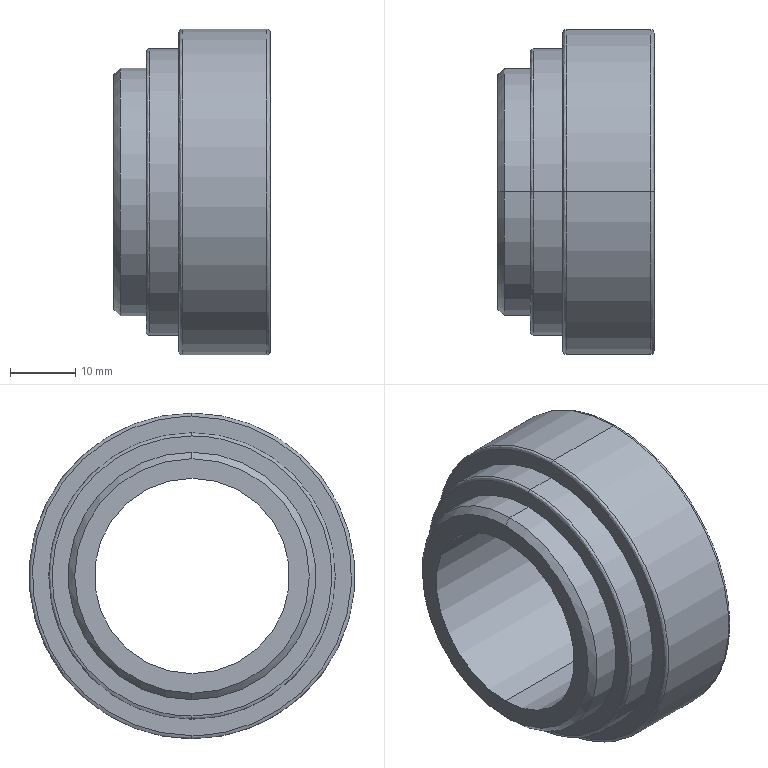Part | SolidWorks | features BaseBody 1 | 1 solid | 22 faces | box 24 x 50 x 50 mm | volume 23661 mm3 | cylinder 8 | spline 6 | cone 4 | plane 4 | commonest cylinder face diameters 30 x2 38 x2 44 x2 50 x2
STEP:
#1=CARTESIAN_POINT('',(-0.5,0.,25.));
#2=VERTEX_POINT('',#1);
#3=CARTESIAN_POINT('',(-0.5,0.,-25.));
#4=VERTEX_POINT('',#3);
#5=CARTESIAN_POINT('',(-0.5,0.,0.));
#6=DIRECTION('',(1.,0.,0.));
#7=DIRECTION('',(0.,0.,1.));
#8=AXIS2_PLACEMENT_3D('',#5,#6,#7);
#9=CIRCLE('',#8,25.);
#10=EDGE_CURVE('',#2,#4,#9,.T.);
#11=ORIENTED_EDGE('',*,*,#10,.T.);
#12=CARTESIAN_POINT('',(0.,0.,-24.5));
#13=VERTEX_POINT('',#12);
#14=CARTESIAN_POINT('',(-0.5,0.,-24.5));
#15=DIRECTION('',(0.,-1.,0.));
#16=DIRECTION('',(0.,0.,-1.));
#17=AXIS2_PLACEMENT_3D('',#14,#15,#16);
#18=CIRCLE('',#17,0.5);
#19=EDGE_CURVE('',#4,#13,#18,.T.);
#20=ORIENTED_EDGE('',*,*,#19,.T.);
#21=CARTESIAN_POINT('',(0.,0.,24.5));
#22=VERTEX_POINT('',#21);
#23=CARTESIAN_POINT('',(0.,0.,24.5));
#24=CARTESIAN_POINT('',(0.,-0.7494,24.5));
#25=CARTESIAN_POINT('',(0.,-1.869,24.449));
#26=CARTESIAN_POINT('',(0.,-3.166,24.3));
#27=CARTESIAN_POINT('',(0.,-3.813,24.203));
#28=CARTESIAN_POINT('',(0.,-4.136,24.149));
#29=CARTESIAN_POINT('',(0.,-4.297,24.12));
#30=CARTESIAN_POINT('',(0.,-4.366,24.108));
#31=CARTESIAN_POINT('',(0.,-4.412,24.099));
#32=CARTESIAN_POINT('',(0.,-4.434,24.095));
#33=CARTESIAN_POINT('',(0.,-5.239,23.946));
#34=CARTESIAN_POINT('',(0.,-6.395,23.674));
#35=CARTESIAN_POINT('',(0.,-7.716,23.259));
#36=CARTESIAN_POINT('',(0.,-8.369,23.028));
#37=CARTESIAN_POINT('',(0.,-8.694,22.906));
#38=CARTESIAN_POINT('',(0.,-8.833,22.852));
#39=CARTESIAN_POINT('',(0.,-8.926,22.816));
#40=CARTESIAN_POINT('',(0.,-8.97,22.799));
#41=CARTESIAN_POINT('',(0.,-9.788,22.475));
#42=CARTESIAN_POINT('',(0.,-10.914,21.962));
#43=CARTESIAN_POINT('',(0.,-12.177,21.267));
#44=CARTESIAN_POINT('',(0.,-12.796,20.895));
#45=CARTESIAN_POINT('',(0.,-13.059,20.73));
#46=CARTESIAN_POINT('',(0.,-13.233,20.619));
#47=CARTESIAN_POINT('',(0.,-13.318,20.564));
#48=CARTESIAN_POINT('',(0.,-14.822,19.581));
#49=CARTESIAN_POINT('',(0.,-16.128,18.52));
#50=CARTESIAN_POINT('',(0.,-17.922,16.726));
#51=CARTESIAN_POINT('',(0.,-18.768,15.788));
#52=CARTESIAN_POINT('',(0.,-19.667,14.622));
#53=CARTESIAN_POINT('',(0.,-20.094,14.02));
#54=CARTESIAN_POINT('',(0.,-20.302,13.715));
#55=CARTESIAN_POINT('',(0.,-20.39,13.583));
#56=CARTESIAN_POINT('',(0.,-20.448,13.495));
#57=CARTESIAN_POINT('',(0.,-20.478,13.45));
#58=CARTESIAN_POINT('',(0.,-20.959,12.714));
#59=CARTESIAN_POINT('',(0.,-21.583,11.646));
#60=CARTESIAN_POINT('',(0.,-22.214,10.349));
#61=CARTESIAN_POINT('',(0.,-22.505,9.688));
#62=CARTESIAN_POINT('',(0.,-22.644,9.354));
#63=CARTESIAN_POINT('',(0.,-22.703,9.21));
#64=CARTESIAN_POINT('',(0.,-22.742,9.114));
#65=CARTESIAN_POINT('',(0.,-22.762,9.064));
#66=CARTESIAN_POINT('',(0.,-23.072,8.28));
#67=CARTESIAN_POINT('',(0.,-23.455,7.156));
#68=CARTESIAN_POINT('',(0.,-23.806,5.816));
#69=CARTESIAN_POINT('',(0.,-23.956,5.14));
#70=CARTESIAN_POINT('',(0.,-24.026,4.799));
#71=CARTESIAN_POINT('',(0.,-24.059,4.629));
#72=CARTESIAN_POINT('',(0.,-24.073,4.556));
#73=CARTESIAN_POINT('',(0.,-24.082,4.507));
#74=CARTESIAN_POINT('',(0.,-24.087,4.481));
#75=CARTESIAN_POINT('',(0.,-24.364,2.985));
#76=CARTESIAN_POINT('',(0.,-24.5,1.498));
#77=CARTESIAN_POINT('',(0.,-24.5,-0.7491));
#78=CARTESIAN_POINT('',(0.,-24.449,-1.868));
#79=CARTESIAN_POINT('',(0.,-24.3,-3.166));
#80=CARTESIAN_POINT('',(0.,-24.203,-3.813));
#81=CARTESIAN_POINT('',(0.,-24.149,-4.136));
#82=CARTESIAN_POINT('',(0.,-24.12,-4.297));
#83=CARTESIAN_POINT('',(0.,-24.108,-4.366));
#84=CARTESIAN_POINT('',(0.,-24.099,-4.412));
#85=CARTESIAN_POINT('',(0.,-24.095,-4.434));
#86=CARTESIAN_POINT('',(0.,-23.946,-5.239));
#87=CARTESIAN_POINT('',(0.,-23.674,-6.395));
#88=CARTESIAN_POINT('',(0.,-23.259,-7.716));
#89=CARTESIAN_POINT('',(0.,-23.028,-8.369));
#90=CARTESIAN_POINT('',(0.,-22.906,-8.694));
#91=CARTESIAN_POINT('',(0.,-22.852,-8.833));
#92=CARTESIAN_POINT('',(0.,-22.816,-8.926));
#93=CARTESIAN_POINT('',(0.,-22.799,-8.97));
#94=CARTESIAN_POINT('',(0.,-22.475,-9.788));
#95=CARTESIAN_POINT('',(0.,-21.962,-10.914));
#96=CARTESIAN_POINT('',(0.,-21.267,-12.177));
#97=CARTESIAN_POINT('',(0.,-20.895,-12.796));
#98=CARTESIAN_POINT('',(0.,-20.73,-13.059));
#99=CARTESIAN_POINT('',(0.,-20.619,-13.233));
#100=CARTESIAN_POINT('',(0.,-20.564,-13.318));
#101=CARTESIAN_POINT('',(0.,-19.581,-14.822));
#102=CARTESIAN_POINT('',(0.,-18.52,-16.128));
#103=CARTESIAN_POINT('',(0.,-16.726,-17.922));
#104=CARTESIAN_POINT('',(0.,-15.788,-18.768));
#105=CARTESIAN_POINT('',(0.,-14.622,-19.667));
#106=CARTESIAN_POINT('',(0.,-14.02,-20.094));
#107=CARTESIAN_POINT('',(0.,-13.715,-20.302));
#108=CARTESIAN_POINT('',(0.,-13.583,-20.39));
#109=CARTESIAN_POINT('',(0.,-13.495,-20.448));
#110=CARTESIAN_POINT('',(0.,-13.45,-20.478));
#111=CARTESIAN_POINT('',(0.,-12.714,-20.959));
#112=CARTESIAN_POINT('',(0.,-11.646,-21.583));
#113=CARTESIAN_POINT('',(0.,-10.349,-22.214));
#114=CARTESIAN_POINT('',(0.,-9.688,-22.505));
#115=CARTESIAN_POINT('',(0.,-9.354,-22.644));
#116=CARTESIAN_POINT('',(0.,-9.21,-22.703));
#117=CARTESIAN_POINT('',(0.,-9.114,-22.742));
#118=CARTESIAN_POINT('',(0.,-9.064,-22.762));
#119=CARTESIAN_POINT('',(0.,-8.28,-23.072));
#120=CARTESIAN_POINT('',(0.,-7.156,-23.455));
#121=CARTESIAN_POINT('',(0.,-5.816,-23.806));
#122=CARTESIAN_POINT('',(0.,-5.14,-23.956));
#123=CARTESIAN_POINT('',(0.,-4.799,-24.026));
#124=CARTESIAN_POINT('',(0.,-4.629,-24.059));
#125=CARTESIAN_POINT('',(0.,-4.556,-24.073));
#126=CARTESIAN_POINT('',(0.,-4.507,-24.082));
#127=CARTESIAN_POINT('',(0.,-4.481,-24.087));
#128=CARTESIAN_POINT('',(0.,-2.985,-24.364));
#129=CARTESIAN_POINT('',(0.,-1.498,-24.5));
#130=CARTESIAN_POINT('',(0.,0.,-24.5));
#131=B_SPLINE_CURVE_WITH_KNOTS('',3,(#23,#24,#25,#26,#27,#28,#29,#30,#31,#32,#33,#34,#35,#36,#37,#38,#39,#40,#41,#42,#43,#44,#45,#46,#47,#48,#49,#50,#51,#52,#53,#54,#55,#56,#57,#58,#59,#60,#61,#62,#63,#64,#65,#66,#67,#68,#69,#70,#71,#72,#73,#74,#75,#76,#77,#78,#79,#80,#81,#82,#83,#84,#85,#86,#87,#88,#89,#90,#91,#92,#93,#94,#95,#96,#97,#98,#99,#100,#101,#102,#103,#104,#105,#106,#107,#108,#109,#110,#111,#112,#113,#114,#115,#116,#117,#118,#119,#120,#121,#122,#123,#124,#125,#126,#127,#128,#129,#130),.UNSPECIFIED.,.F.,.F.,(4,1,1,1,1,1,2,2,1,1,1,1,2,2,1,1,1,2,2,2,1,1,1,1,2,2,1,1,1,1,2,2,1,1,1,1,1,2,2,2,1,1,1,1,1,2,2,1,1,1,1,2,2,1,1,1,2,2,2,1,1,1,1,2,2,1,1,1,1,2,2,1,1,1,1,1,2,2,4),(0.,0.01562,0.02344,0.02734,0.0293,0.03027,0.03076,0.03125,0.04687,0.05469,0.05859,0.06055,0.06152,0.0625,0.07812,0.08594,0.08984,0.0918,0.09375,0.125,0.1406,0.1484,0.1523,0.1543,0.1553,0.1562,0.1719,0.1797,0.1836,0.1855,0.1865,0.1875,0.2031,0.2109,0.2148,0.2168,0.2178,0.2183,0.2187,0.25,0.2656,0.2734,0.2773,0.2793,0.2803,0.2808,0.2812,0.2969,0.3047,0.3086,0.3105,0.3115,0.3125,0.3281,0.3359,0.3398,0.3418,0.3437,0.375,0.3906,0.3984,0.4023,0.4043,0.4053,0.4063,0.4219,0.4297,0.4336,0.4355,0.4365,0.4375,0.4531,0.4609,0.4648,0.4668,0.4678,0.4683,0.4688,0.5),.UNSPECIFIED.);
#132=EDGE_CURVE('',#22,#13,#131,.T.);
#133=ORIENTED_EDGE('',*,*,#132,.F.);
#134=CARTESIAN_POINT('',(-0.5,0.,24.5));
#135=DIRECTION('',(0.,1.,0.));
#136=DIRECTION('',(0.,0.,1.));
#137=AXIS2_PLACEMENT_3D('',#134,#135,#136);
#138=CIRCLE('',#137,0.5);
#139=EDGE_CURVE('',#2,#22,#138,.T.);
#140=ORIENTED_EDGE('',*,*,#139,.F.);
#141=EDGE_LOOP('',(#11,#20,#133,#140));
#142=FACE_OUTER_BOUND('',#141,.T.);
#143=CARTESIAN_POINT('',(-0.5,0.,-25.));
#144=CARTESIAN_POINT('',(-0.5,-50.,-25.));
#145=CARTESIAN_POINT('',(-0.5,-50.,25.));
#146=CARTESIAN_POINT('',(-0.5,0.,25.));
#147=CARTESIAN_POINT('',(-0.2071,0.,-25.));
#148=CARTESIAN_POINT('',(-0.2071,-50.,-25.));
#149=CARTESIAN_POINT('',(-0.2071,-50.,25.));
#150=CARTESIAN_POINT('',(-0.2071,0.,25.));
#151=CARTESIAN_POINT('',(0.,0.,-24.793));
#152=CARTESIAN_POINT('',(0.,-49.586,-24.793));
#153=CARTESIAN_POINT('',(0.,-49.586,24.793));
#154=CARTESIAN_POINT('',(0.,0.,24.793));
#155=CARTESIAN_POINT('',(0.,0.,-24.5));
#156=CARTESIAN_POINT('',(0.,-49.,-24.5));
#157=CARTESIAN_POINT('',(0.,-49.,24.5));
#158=CARTESIAN_POINT('',(0.,0.,24.5));
#159=(BOUNDED_SURFACE()B_SPLINE_SURFACE(3,3,((#143,#144,#145,#146),(#147,#148,#149,#150),(#151,#152,#153,#154),(#155,#156,#157,#158)),.UNSPECIFIED.,.F.,.F.,.F.)B_SPLINE_SURFACE_WITH_KNOTS((4,4),(4,4),(0.,1.),(0.,1.),.UNSPECIFIED.)GEOMETRIC_REPRESENTATION_ITEM()RATIONAL_B_SPLINE_SURFACE(((1.,0.3333,0.3333,1.),(0.8047,0.2682,0.2682,0.8047),(0.8047,0.2682,0.2682,0.8047),(1.,0.3333,0.3333,1.)))REPRESENTATION_ITEM('')SURFACE());
#160=ADVANCED_FACE('',(#142),#159,.T.);
#161=CARTESIAN_POINT('',(-14.,0.,24.5));
#162=VERTEX_POINT('',#161);
#163=CARTESIAN_POINT('',(-14.,0.,-24.5));
#164=VERTEX_POINT('',#163);
#165=CARTESIAN_POINT('',(-14.,0.,24.5));
#166=CARTESIAN_POINT('',(-14.,-49.,24.5));
#167=CARTESIAN_POINT('',(-14.,-49.,-24.5));
#168=CARTESIAN_POINT('',(-14.,0.,-24.5));
#169=(BOUNDED_CURVE()B_SPLINE_CURVE(3,(#165,#166,#167,#168),.UNSPECIFIED.,.F.,.F.)B_SPLINE_CURVE_WITH_KNOTS((4,4),(0.,0.5),.UNSPECIFIED.)CURVE()GEOMETRIC_REPRESENTATION_ITEM()RATIONAL_B_SPLINE_CURVE((1.,0.3333,0.3333,1.))REPRESENTATION_ITEM(''));
#170=EDGE_CURVE('',#162,#164,#169,.T.);
#171=ORIENTED_EDGE('',*,*,#170,.T.);
#172=CARTESIAN_POINT('',(-13.5,0.,-25.));
#173=VERTEX_POINT('',#172);
#174=CARTESIAN_POINT('',(-13.5,0.,-24.5));
#175=DIRECTION('',(0.,-1.,0.));
#176=DIRECTION('',(0.,0.,-1.));
#177=AXIS2_PLACEMENT_3D('',#174,#175,#176);
#178=CIRCLE('',#177,0.5);
#179=EDGE_CURVE('',#164,#173,#178,.T.);
#180=ORIENTED_EDGE('',*,*,#179,.T.);
#181=CARTESIAN_POINT('',(-13.5,0.,25.));
#182=VERTEX_POINT('',#181);
#183=CARTESIAN_POINT('',(-13.5,0.,0.));
#184=DIRECTION('',(1.,0.,0.));
#185=DIRECTION('',(0.,0.,1.));
#186=AXIS2_PLACEMENT_3D('',#183,#184,#185);
#187=CIRCLE('',#186,25.);
#188=EDGE_CURVE('',#182,#173,#187,.T.);
#189=ORIENTED_EDGE('',*,*,#188,.F.);
#190=CARTESIAN_POINT('',(-13.5,0.,24.5));
#191=DIRECTION('',(0.,1.,0.));
#192=DIRECTION('',(0.,0.,1.));
#193=AXIS2_PLACEMENT_3D('',#190,#191,#192);
#194=CIRCLE('',#193,0.5);
#195=EDGE_CURVE('',#162,#182,#194,.T.);
#196=ORIENTED_EDGE('',*,*,#195,.F.);
#197=EDGE_LOOP('',(#171,#180,#189,#196));
#198=FACE_OUTER_BOUND('',#197,.T.);
#199=CARTESIAN_POINT('',(-14.,0.,-24.5));
#200=CARTESIAN_POINT('',(-14.,-49.,-24.5));
#201=CARTESIAN_POINT('',(-14.,-49.,24.5));
#202=CARTESIAN_POINT('',(-14.,0.,24.5));
#203=CARTESIAN_POINT('',(-14.,0.,-24.793));
#204=CARTESIAN_POINT('',(-14.,-49.586,-24.793));
#205=CARTESIAN_POINT('',(-14.,-49.586,24.793));
#206=CARTESIAN_POINT('',(-14.,0.,24.793));
#207=CARTESIAN_POINT('',(-13.793,0.,-25.));
#208=CARTESIAN_POINT('',(-13.793,-50.,-25.));
#209=CARTESIAN_POINT('',(-13.793,-50.,25.));
#210=CARTESIAN_POINT('',(-13.793,0.,25.));
#211=CARTESIAN_POINT('',(-13.5,0.,-25.));
#212=CARTESIAN_POINT('',(-13.5,-50.,-25.));
#213=CARTESIAN_POINT('',(-13.5,-50.,25.));
#214=CARTESIAN_POINT('',(-13.5,0.,25.));
#215=(BOUNDED_SURFACE()B_SPLINE_SURFACE(3,3,((#199,#200,#201,#202),(#203,#204,#205,#206),(#207,#208,#209,#210),(#211,#212,#213,#214)),.UNSPECIFIED.,.F.,.F.,.F.)B_SPLINE_SURFACE_WITH_KNOTS((4,4),(4,4),(0.,1.),(0.,1.),.UNSPECIFIED.)GEOMETRIC_REPRESENTATION_ITEM()RATIONAL_B_SPLINE_SURFACE(((1.,0.3333,0.3333,1.),(0.8047,0.2682,0.2682,0.8047),(0.8047,0.2682,0.2682,0.8047),(1.,0.3333,0.3333,1.)))REPRESENTATION_ITEM('')SURFACE());
#216=ADVANCED_FACE('',(#198),#215,.T.);
#217=CARTESIAN_POINT('',(-19.,0.,-21.5));
#218=VERTEX_POINT('',#217);
#219=CARTESIAN_POINT('',(-19.,0.,21.5));
#220=VERTEX_POINT('',#219);
#221=CARTESIAN_POINT('',(-19.,0.,-21.5));
#222=CARTESIAN_POINT('',(-19.,-0.6573,-21.5));
#223=CARTESIAN_POINT('',(-19.,-1.639,-21.455));
#224=CARTESIAN_POINT('',(-19.,-2.778,-21.324));
#225=CARTESIAN_POINT('',(-19.,-3.346,-21.239));
#226=CARTESIAN_POINT('',(-19.,-3.629,-21.192));
#227=CARTESIAN_POINT('',(-19.,-3.771,-21.167));
#228=CARTESIAN_POINT('',(-19.,-3.831,-21.156));
#229=CARTESIAN_POINT('',(-19.,-3.872,-21.149));
#230=CARTESIAN_POINT('',(-19.,-3.891,-21.145));
#231=CARTESIAN_POINT('',(-19.,-4.598,-21.014));
#232=CARTESIAN_POINT('',(-19.,-5.612,-20.775));
#233=CARTESIAN_POINT('',(-19.,-6.771,-20.411));
#234=CARTESIAN_POINT('',(-19.,-7.345,-20.208));
#235=CARTESIAN_POINT('',(-19.,-7.63,-20.101));
#236=CARTESIAN_POINT('',(-19.,-7.752,-20.054));
#237=CARTESIAN_POINT('',(-19.,-7.833,-20.022));
#238=CARTESIAN_POINT('',(-19.,-7.872,-20.007));
#239=CARTESIAN_POINT('',(-19.,-8.589,-19.723));
#240=CARTESIAN_POINT('',(-19.,-9.577,-19.273));
#241=CARTESIAN_POINT('',(-19.,-10.686,-18.663));
#242=CARTESIAN_POINT('',(-19.,-11.229,-18.336));
#243=CARTESIAN_POINT('',(-19.,-11.46,-18.192));
#244=CARTESIAN_POINT('',(-19.,-11.613,-18.094));
#245=CARTESIAN_POINT('',(-19.,-11.687,-18.046));
#246=CARTESIAN_POINT('',(-19.,-13.007,-17.183));
#247=CARTESIAN_POINT('',(-19.,-14.153,-16.252));
#248=CARTESIAN_POINT('',(-19.,-15.727,-14.678));
#249=CARTESIAN_POINT('',(-19.,-16.47,-13.855));
#250=CARTESIAN_POINT('',(-19.,-17.259,-12.831));
#251=CARTESIAN_POINT('',(-19.,-17.633,-12.303));
#252=CARTESIAN_POINT('',(-19.,-17.79,-12.074));
#253=CARTESIAN_POINT('',(-19.,-17.893,-11.92));
#254=CARTESIAN_POINT('',(-19.,-17.946,-11.841));
#255=CARTESIAN_POINT('',(-19.,-18.393,-11.157));
#256=CARTESIAN_POINT('',(-19.,-18.94,-10.22));
#257=CARTESIAN_POINT('',(-19.,-19.494,-9.082));
#258=CARTESIAN_POINT('',(-19.,-19.749,-8.502));
#259=CARTESIAN_POINT('',(-19.,-19.872,-8.209));
#260=CARTESIAN_POINT('',(-19.,-19.923,-8.083));
#261=CARTESIAN_POINT('',(-19.,-19.957,-7.998));
#262=CARTESIAN_POINT('',(-19.,-19.974,-7.955));
#263=CARTESIAN_POINT('',(-19.,-20.247,-7.266));
#264=CARTESIAN_POINT('',(-19.,-20.583,-6.28));
#265=CARTESIAN_POINT('',(-19.,-20.891,-5.104));
#266=CARTESIAN_POINT('',(-19.,-21.023,-4.51));
#267=CARTESIAN_POINT('',(-19.,-21.084,-4.212));
#268=CARTESIAN_POINT('',(-19.,-21.113,-4.062));
#269=CARTESIAN_POINT('',(-19.,-21.125,-3.998));
#270=CARTESIAN_POINT('',(-19.,-21.133,-3.955));
#271=CARTESIAN_POINT('',(-19.,-21.137,-3.932));
#272=CARTESIAN_POINT('',(-19.,-21.38,-2.619));
#273=CARTESIAN_POINT('',(-19.,-21.5,-1.315));
#274=CARTESIAN_POINT('',(-19.,-21.5,0.6573));
#275=CARTESIAN_POINT('',(-19.,-21.455,1.639));
#276=CARTESIAN_POINT('',(-19.,-21.324,2.778));
#277=CARTESIAN_POINT('',(-19.,-21.239,3.346));
#278=CARTESIAN_POINT('',(-19.,-21.192,3.629));
#279=CARTESIAN_POINT('',(-19.,-21.167,3.771));
#280=CARTESIAN_POINT('',(-19.,-21.156,3.831));
#281=CARTESIAN_POINT('',(-19.,-21.149,3.872));
#282=CARTESIAN_POINT('',(-19.,-21.145,3.891));
#283=CARTESIAN_POINT('',(-19.,-21.014,4.598));
#284=CARTESIAN_POINT('',(-19.,-20.775,5.612));
#285=CARTESIAN_POINT('',(-19.,-20.411,6.771));
#286=CARTESIAN_POINT('',(-19.,-20.208,7.345));
#287=CARTESIAN_POINT('',(-19.,-20.101,7.63));
#288=CARTESIAN_POINT('',(-19.,-20.054,7.752));
#289=CARTESIAN_POINT('',(-19.,-20.022,7.833));
#290=CARTESIAN_POINT('',(-19.,-20.007,7.872));
#291=CARTESIAN_POINT('',(-19.,-19.723,8.589));
#292=CARTESIAN_POINT('',(-19.,-19.273,9.577));
#293=CARTESIAN_POINT('',(-19.,-18.663,10.686));
#294=CARTESIAN_POINT('',(-19.,-18.336,11.229));
#295=CARTESIAN_POINT('',(-19.,-18.192,11.46));
#296=CARTESIAN_POINT('',(-19.,-18.094,11.613));
#297=CARTESIAN_POINT('',(-19.,-18.046,11.687));
#298=CARTESIAN_POINT('',(-19.,-17.183,13.007));
#299=CARTESIAN_POINT('',(-19.,-16.252,14.153));
#300=CARTESIAN_POINT('',(-19.,-14.678,15.727));
#301=CARTESIAN_POINT('',(-19.,-13.855,16.47));
#302=CARTESIAN_POINT('',(-19.,-12.831,17.259));
#303=CARTESIAN_POINT('',(-19.,-12.303,17.633));
#304=CARTESIAN_POINT('',(-19.,-12.074,17.79));
#305=CARTESIAN_POINT('',(-19.,-11.92,17.893));
#306=CARTESIAN_POINT('',(-19.,-11.841,17.946));
#307=CARTESIAN_POINT('',(-19.,-11.157,18.393));
#308=CARTESIAN_POINT('',(-19.,-10.22,18.94));
#309=CARTESIAN_POINT('',(-19.,-9.082,19.494));
#310=CARTESIAN_POINT('',(-19.,-8.502,19.749));
#311=CARTESIAN_POINT('',(-19.,-8.209,19.872));
#312=CARTESIAN_POINT('',(-19.,-8.083,19.923));
#313=CARTESIAN_POINT('',(-19.,-7.998,19.957));
#314=CARTESIAN_POINT('',(-19.,-7.955,19.974));
#315=CARTESIAN_POINT('',(-19.,-7.266,20.247));
#316=CARTESIAN_POINT('',(-19.,-6.28,20.583));
#317=CARTESIAN_POINT('',(-19.,-5.104,20.891));
#318=CARTESIAN_POINT('',(-19.,-4.51,21.023));
#319=CARTESIAN_POINT('',(-19.,-4.212,21.084));
#320=CARTESIAN_POINT('',(-19.,-4.062,21.113));
#321=CARTESIAN_POINT('',(-19.,-3.998,21.125));
#322=CARTESIAN_POINT('',(-19.,-3.955,21.133));
#323=CARTESIAN_POINT('',(-19.,-3.932,21.137));
#324=CARTESIAN_POINT('',(-19.,-2.619,21.38));
#325=CARTESIAN_POINT('',(-19.,-1.315,21.5));
#326=CARTESIAN_POINT('',(-19.,0.,21.5));
#327=B_SPLINE_CURVE_WITH_KNOTS('',3,(#221,#222,#223,#224,#225,#226,#227,#228,#229,#230,#231,#232,#233,#234,#235,#236,#237,#238,#239,#240,#241,#242,#243,#244,#245,#246,#247,#248,#249,#250,#251,#252,#253,#254,#255,#256,#257,#258,#259,#260,#261,#262,#263,#264,#265,#266,#267,#268,#269,#270,#271,#272,#273,#274,#275,#276,#277,#278,#279,#280,#281,#282,#283,#284,#285,#286,#287,#288,#289,#290,#291,#292,#293,#294,#295,#296,#297,#298,#299,#300,#301,#302,#303,#304,#305,#306,#307,#308,#309,#310,#311,#312,#313,#314,#315,#316,#317,#318,#319,#320,#321,#322,#323,#324,#325,#326),.UNSPECIFIED.,.F.,.F.,(4,1,1,1,1,1,2,2,1,1,1,1,2,2,1,1,1,2,2,2,1,1,1,2,2,1,1,1,1,2,2,1,1,1,1,1,2,2,2,1,1,1,1,1,2,2,1,1,1,1,2,2,1,1,1,2,2,2,1,1,1,2,2,1,1,1,1,2,2,1,1,1,1,1,2,2,4),(0.5,0.5156,0.5234,0.5273,0.5293,0.5303,0.5308,0.5313,0.5469,0.5547,0.5586,0.5605,0.5615,0.5625,0.5781,0.5859,0.5898,0.5918,0.5938,0.625,0.6406,0.6484,0.6523,0.6543,0.6563,0.6719,0.6797,0.6836,0.6855,0.6865,0.6875,0.7031,0.7109,0.7148,0.7168,0.7178,0.7183,0.7188,0.75,0.7656,0.7734,0.7773,0.7793,0.7803,0.7808,0.7813,0.7969,0.8047,0.8086,0.8105,0.8115,0.8125,0.8281,0.8359,0.8398,0.8418,0.8438,0.875,0.8906,0.8984,0.9023,0.9043,0.9063,0.9219,0.9297,0.9336,0.9355,0.9365,0.9375,0.9531,0.9609,0.9648,0.9668,0.9678,0.9683,0.9688,1.),.UNSPECIFIED.);
#328=EDGE_CURVE('',#218,#220,#327,.T.);
#329=ORIENTED_EDGE('',*,*,#328,.F.);
#330=CARTESIAN_POINT('',(-18.5,0.,-22.));
#331=VERTEX_POINT('',#330);
#332=CARTESIAN_POINT('',(-18.5,0.,-21.5));
#333=DIRECTION('',(0.,-1.,0.));
#334=DIRECTION('',(0.,0.,-1.));
#335=AXIS2_PLACEMENT_3D('',#332,#333,#334);
#336=CIRCLE('',#335,0.5);
#337=EDGE_CURVE('',#218,#331,#336,.T.);
#338=ORIENTED_EDGE('',*,*,#337,.T.);
#339=CARTESIAN_POINT('',(-18.5,0.,22.));
#340=VERTEX_POINT('',#339);
#341=CARTESIAN_POINT('',(-18.5,0.,0.));
#342=DIRECTION('',(-1.,0.,0.));
#343=DIRECTION('',(0.,0.,1.));
#344=AXIS2_PLACEMENT_3D('',#341,#342,#343);
#345=CIRCLE('',#344,22.);
#346=EDGE_CURVE('',#331,#340,#345,.T.);
#347=ORIENTED_EDGE('',*,*,#346,.T.);
#348=CARTESIAN_POINT('',(-18.5,0.,21.5));
#349=DIRECTION('',(0.,1.,0.));
#350=DIRECTION('',(0.,0.,1.));
#351=AXIS2_PLACEMENT_3D('',#348,#349,#350);
#352=CIRCLE('',#351,0.5);
#353=EDGE_CURVE('',#220,#340,#352,.T.);
#354=ORIENTED_EDGE('',*,*,#353,.F.);
#355=EDGE_LOOP('',(#329,#338,#347,#354));
#356=FACE_OUTER_BOUND('',#355,.T.);
#357=CARTESIAN_POINT('',(-19.,0.,-21.5));
#358=CARTESIAN_POINT('',(-19.,-43.,-21.5));
#359=CARTESIAN_POINT('',(-19.,-43.,21.5));
#360=CARTESIAN_POINT('',(-19.,0.,21.5));
#361=CARTESIAN_POINT('',(-19.,0.,-21.793));
#362=CARTESIAN_POINT('',(-19.,-43.586,-21.793));
#363=CARTESIAN_POINT('',(-19.,-43.586,21.793));
#364=CARTESIAN_POINT('',(-19.,0.,21.793));
#365=CARTESIAN_POINT('',(-18.793,0.,-22.));
#366=CARTESIAN_POINT('',(-18.793,-44.,-22.));
#367=CARTESIAN_POINT('',(-18.793,-44.,22.));
#368=CARTESIAN_POINT('',(-18.793,0.,22.));
#369=CARTESIAN_POINT('',(-18.5,0.,-22.));
#370=CARTESIAN_POINT('',(-18.5,-44.,-22.));
#371=CARTESIAN_POINT('',(-18.5,-44.,22.));
#372=CARTESIAN_POINT('',(-18.5,0.,22.));
#373=(BOUNDED_SURFACE()B_SPLINE_SURFACE(3,3,((#357,#358,#359,#360),(#361,#362,#363,#364),(#365,#366,#367,#368),(#369,#370,#371,#372)),.UNSPECIFIED.,.F.,.F.,.F.)B_SPLINE_SURFACE_WITH_KNOTS((4,4),(4,4),(0.,1.),(0.,1.),.UNSPECIFIED.)GEOMETRIC_REPRESENTATION_ITEM()RATIONAL_B_SPLINE_SURFACE(((1.,0.3333,0.3333,1.),(0.8047,0.2682,0.2682,0.8047),(0.8047,0.2682,0.2682,0.8047),(1.,0.3333,0.3333,1.)))REPRESENTATION_ITEM('')SURFACE());
#374=ADVANCED_FACE('',(#356),#373,.T.);
#375=CARTESIAN_POINT('',(-1.,0.,-15.));
#376=VERTEX_POINT('',#375);
#377=CARTESIAN_POINT('',(-1.,0.,15.));
#378=VERTEX_POINT('',#377);
#379=CARTESIAN_POINT('',(-1.,0.,0.));
#380=DIRECTION('',(-1.,0.,0.));
#381=DIRECTION('',(0.,0.,1.));
#382=AXIS2_PLACEMENT_3D('',#379,#380,#381);
#383=CIRCLE('',#382,15.);
#384=EDGE_CURVE('',#376,#378,#383,.T.);
#385=ORIENTED_EDGE('',*,*,#384,.F.);
#386=CARTESIAN_POINT('',(-24.,0.,-15.));
#387=VERTEX_POINT('',#386);
#388=CARTESIAN_POINT('',(0.,0.,-15.));
#389=DIRECTION('',(-1.,0.,0.));
#390=VECTOR('',#389,1000.);
#391=LINE('',#388,#390);
#392=EDGE_CURVE('',#376,#387,#391,.T.);
#393=ORIENTED_EDGE('',*,*,#392,.T.);
#394=CARTESIAN_POINT('',(-24.,0.,15.));
#395=VERTEX_POINT('',#394);
#396=CARTESIAN_POINT('',(-24.,0.,0.));
#397=DIRECTION('',(1.,0.,0.));
#398=DIRECTION('',(0.,0.,1.));
#399=AXIS2_PLACEMENT_3D('',#396,#397,#398);
#400=CIRCLE('',#399,15.);
#401=EDGE_CURVE('',#395,#387,#400,.T.);
#402=ORIENTED_EDGE('',*,*,#401,.F.);
#403=CARTESIAN_POINT('',(0.,0.,15.));
#404=DIRECTION('',(-1.,0.,0.));
#405=VECTOR('',#404,1000.);
#406=LINE('',#403,#405);
#407=EDGE_CURVE('',#378,#395,#406,.T.);
#408=ORIENTED_EDGE('',*,*,#407,.F.);
#409=EDGE_LOOP('',(#385,#393,#402,#408));
#410=FACE_OUTER_BOUND('',#409,.T.);
#411=CARTESIAN_POINT('',(0.,0.,0.));
#412=DIRECTION('',(-1.,0.,0.));
#413=DIRECTION('',(0.,0.,1.));
#414=AXIS2_PLACEMENT_3D('',#411,#412,#413);
#415=CYLINDRICAL_SURFACE('',#414,15.);
#416=ADVANCED_FACE('',(#410),#415,.F.);
#417=ORIENTED_EDGE('',*,*,#384,.T.);
#418=CARTESIAN_POINT('',(0.,0.,16.));
#419=VERTEX_POINT('',#418);
#420=CARTESIAN_POINT('',(0.,0.,16.));
#421=DIRECTION('',(0.7071,0.,0.7071));
#422=VECTOR('',#421,1000.);
#423=LINE('',#420,#422);
#424=EDGE_CURVE('',#378,#419,#423,.T.);
#425=ORIENTED_EDGE('',*,*,#424,.T.);
#426=CARTESIAN_POINT('',(0.,0.,-16.));
#427=VERTEX_POINT('',#426);
#428=CARTESIAN_POINT('',(0.,0.,0.));
#429=DIRECTION('',(-1.,0.,0.));
#430=DIRECTION('',(0.,0.,-1.));
#431=AXIS2_PLACEMENT_3D('',#428,#429,#430);
#432=CIRCLE('',#431,16.);
#433=EDGE_CURVE('',#427,#419,#432,.T.);
#434=ORIENTED_EDGE('',*,*,#433,.F.);
#435=CARTESIAN_POINT('',(0.,0.,-16.));
#436=DIRECTION('',(0.7071,0.,-0.7071));
#437=VECTOR('',#436,1000.);
#438=LINE('',#435,#437);
#439=EDGE_CURVE('',#376,#427,#438,.T.);
#440=ORIENTED_EDGE('',*,*,#439,.F.);
#441=EDGE_LOOP('',(#417,#425,#434,#440));
#442=FACE_OUTER_BOUND('',#441,.T.);
#443=CARTESIAN_POINT('',(0.,0.,0.));
#444=DIRECTION('',(1.,0.,0.));
#445=DIRECTION('',(0.,0.,-1.));
#446=AXIS2_PLACEMENT_3D('',#443,#444,#445);
#447=CONICAL_SURFACE('',#446,16.,0.7854);
#448=ADVANCED_FACE('',(#442),#447,.F.);
#449=CARTESIAN_POINT('',(-24.,0.,18.));
#450=VERTEX_POINT('',#449);
#451=CARTESIAN_POINT('',(-24.,0.,-18.));
#452=VERTEX_POINT('',#451);
#453=CARTESIAN_POINT('',(-24.,0.,0.));
#454=DIRECTION('',(-1.,0.,0.));
#455=DIRECTION('',(0.,0.,-1.));
#456=AXIS2_PLACEMENT_3D('',#453,#454,#455);
#457=CIRCLE('',#456,18.);
#458=EDGE_CURVE('',#450,#452,#457,.T.);
#459=ORIENTED_EDGE('',*,*,#458,.F.);
#460=CARTESIAN_POINT('',(-23.,0.,19.));
#461=VERTEX_POINT('',#460);
#462=CARTESIAN_POINT('',(-23.,0.,19.));
#463=DIRECTION('',(0.7071,0.,0.7071));
#464=VECTOR('',#463,1000.);
#465=LINE('',#462,#464);
#466=EDGE_CURVE('',#450,#461,#465,.T.);
#467=ORIENTED_EDGE('',*,*,#466,.T.);
#468=CARTESIAN_POINT('',(-23.,0.,-19.));
#469=VERTEX_POINT('',#468);
#470=CARTESIAN_POINT('',(-23.,0.,0.));
#471=DIRECTION('',(-1.,0.,0.));
#472=DIRECTION('',(0.,0.,-1.));
#473=AXIS2_PLACEMENT_3D('',#470,#471,#472);
#474=CIRCLE('',#473,19.);
#475=EDGE_CURVE('',#461,#469,#474,.T.);
#476=ORIENTED_EDGE('',*,*,#475,.T.);
#477=CARTESIAN_POINT('',(-23.,0.,-19.));
#478=DIRECTION('',(0.7071,0.,-0.7071));
#479=VECTOR('',#478,1000.);
#480=LINE('',#477,#479);
#481=EDGE_CURVE('',#452,#469,#480,.T.);
#482=ORIENTED_EDGE('',*,*,#481,.F.);
#483=EDGE_LOOP('',(#459,#467,#476,#482));
#484=FACE_OUTER_BOUND('',#483,.T.);
#485=CARTESIAN_POINT('',(-23.,0.,0.));
#486=DIRECTION('',(1.,0.,0.));
#487=DIRECTION('',(0.,0.,-1.));
#488=AXIS2_PLACEMENT_3D('',#485,#486,#487);
#489=CONICAL_SURFACE('',#488,19.,0.7854);
#490=ADVANCED_FACE('',(#484),#489,.T.);
#491=CARTESIAN_POINT('',(-19.,0.,19.));
#492=VERTEX_POINT('',#491);
#493=CARTESIAN_POINT('',(-19.,0.,-19.));
#494=VERTEX_POINT('',#493);
#495=CARTESIAN_POINT('',(-19.,0.,0.));
#496=DIRECTION('',(-1.,0.,0.));
#497=DIRECTION('',(0.,0.,1.));
#498=AXIS2_PLACEMENT_3D('',#495,#496,#497);
#499=CIRCLE('',#498,19.);
#500=EDGE_CURVE('',#492,#494,#499,.T.);
#501=ORIENTED_EDGE('',*,*,#500,.T.);
#502=CARTESIAN_POINT('',(-21.5,0.,-19.));
#503=DIRECTION('',(-1.,0.,0.));
#504=VECTOR('',#503,1000.);
#505=LINE('',#502,#504);
#506=EDGE_CURVE('',#494,#469,#505,.T.);
#507=ORIENTED_EDGE('',*,*,#506,.T.);
#508=ORIENTED_EDGE('',*,*,#475,.F.);
#509=CARTESIAN_POINT('',(-21.5,0.,19.));
#510=DIRECTION('',(-1.,0.,0.));
#511=VECTOR('',#510,1000.);
#512=LINE('',#509,#511);
#513=EDGE_CURVE('',#492,#461,#512,.T.);
#514=ORIENTED_EDGE('',*,*,#513,.F.);
#515=EDGE_LOOP('',(#501,#507,#508,#514));
#516=FACE_OUTER_BOUND('',#515,.T.);
#517=CARTESIAN_POINT('',(-21.5,0.,0.));
#518=DIRECTION('',(-1.,0.,0.));
#519=DIRECTION('',(0.,0.,1.));
#520=AXIS2_PLACEMENT_3D('',#517,#518,#519);
#521=CYLINDRICAL_SURFACE('',#520,19.);
#522=ADVANCED_FACE('',(#516),#521,.T.);
#523=CARTESIAN_POINT('',(-0.5,0.,0.));
#524=DIRECTION('',(1.,0.,0.));
#525=DIRECTION('',(0.,0.,1.));
#526=AXIS2_PLACEMENT_3D('',#523,#524,#525);
#527=CIRCLE('',#526,25.);
#528=EDGE_CURVE('',#4,#2,#527,.T.);
#529=ORIENTED_EDGE('',*,*,#528,.F.);
#530=CARTESIAN_POINT('',(-7.,0.,-25.));
#531=DIRECTION('',(-1.,0.,0.));
#532=VECTOR('',#531,1000.);
#533=LINE('',#530,#532);
#534=EDGE_CURVE('',#4,#173,#533,.T.);
#535=ORIENTED_EDGE('',*,*,#534,.T.);
#536=CARTESIAN_POINT('',(-13.5,0.,0.));
#537=DIRECTION('',(1.,0.,0.));
#538=DIRECTION('',(0.,0.,1.));
#539=AXIS2_PLACEMENT_3D('',#536,#537,#538);
#540=CIRCLE('',#539,25.);
#541=EDGE_CURVE('',#173,#182,#540,.T.);
#542=ORIENTED_EDGE('',*,*,#541,.T.);
#543=CARTESIAN_POINT('',(-7.,0.,25.));
#544=DIRECTION('',(-1.,0.,0.));
#545=VECTOR('',#544,1000.);
#546=LINE('',#543,#545);
#547=EDGE_CURVE('',#2,#182,#546,.T.);
#548=ORIENTED_EDGE('',*,*,#547,.F.);
#549=EDGE_LOOP('',(#529,#535,#542,#548));
#550=FACE_OUTER_BOUND('',#549,.T.);
#551=CARTESIAN_POINT('',(-7.,0.,0.));
#552=DIRECTION('',(-1.,0.,0.));
#553=DIRECTION('',(0.,0.,1.));
#554=AXIS2_PLACEMENT_3D('',#551,#552,#553);
#555=CYLINDRICAL_SURFACE('',#554,25.);
#556=ADVANCED_FACE('',(#550),#555,.T.);
#557=CARTESIAN_POINT('',(-14.,0.,-22.));
#558=VERTEX_POINT('',#557);
#559=CARTESIAN_POINT('',(-14.,0.,22.));
#560=VERTEX_POINT('',#559);
#561=CARTESIAN_POINT('',(-14.,0.,0.));
#562=DIRECTION('',(1.,0.,0.));
#563=DIRECTION('',(0.,0.,1.));
#564=AXIS2_PLACEMENT_3D('',#561,#562,#563);
#565=CIRCLE('',#564,22.);
#566=EDGE_CURVE('',#558,#560,#565,.T.);
#567=ORIENTED_EDGE('',*,*,#566,.F.);
#568=CARTESIAN_POINT('',(-16.5,0.,-22.));
#569=DIRECTION('',(-1.,0.,0.));
#570=VECTOR('',#569,1000.);
#571=LINE('',#568,#570);
#572=EDGE_CURVE('',#558,#331,#571,.T.);
#573=ORIENTED_EDGE('',*,*,#572,.T.);
#574=CARTESIAN_POINT('',(-18.5,0.,0.));
#575=DIRECTION('',(-1.,0.,0.));
#576=DIRECTION('',(0.,0.,1.));
#577=AXIS2_PLACEMENT_3D('',#574,#575,#576);
#578=CIRCLE('',#577,22.);
#579=EDGE_CURVE('',#340,#331,#578,.T.);
#580=ORIENTED_EDGE('',*,*,#579,.F.);
#581=CARTESIAN_POINT('',(-16.5,0.,22.));
#582=DIRECTION('',(-1.,0.,0.));
#583=VECTOR('',#582,1000.);
#584=LINE('',#581,#583);
#585=EDGE_CURVE('',#560,#340,#584,.T.);
#586=ORIENTED_EDGE('',*,*,#585,.F.);
#587=EDGE_LOOP('',(#567,#573,#580,#586));
#588=FACE_OUTER_BOUND('',#587,.T.);
#589=CARTESIAN_POINT('',(-16.5,0.,0.));
#590=DIRECTION('',(-1.,0.,0.));
#591=DIRECTION('',(0.,0.,1.));
#592=AXIS2_PLACEMENT_3D('',#589,#590,#591);
#593=CYLINDRICAL_SURFACE('',#592,22.);
#594=ADVANCED_FACE('',(#588),#593,.T.);
#595=ORIENTED_EDGE('',*,*,#392,.F.);
#596=CARTESIAN_POINT('',(-1.,0.,0.));
#597=DIRECTION('',(-1.,0.,0.));
#598=DIRECTION('',(0.,0.,1.));
#599=AXIS2_PLACEMENT_3D('',#596,#597,#598);
#600=CIRCLE('',#599,15.);
#601=EDGE_CURVE('',#378,#376,#600,.T.);
#602=ORIENTED_EDGE('',*,*,#601,.F.);
#603=ORIENTED_EDGE('',*,*,#407,.T.);
#604=CARTESIAN_POINT('',(-24.,0.,0.));
#605=DIRECTION('',(1.,0.,0.));
#606=DIRECTION('',(0.,0.,1.));
#607=AXIS2_PLACEMENT_3D('',#604,#605,#606);
#608=CIRCLE('',#607,15.);
#609=EDGE_CURVE('',#387,#395,#608,.T.);
#610=ORIENTED_EDGE('',*,*,#609,.F.);
#611=EDGE_LOOP('',(#595,#602,#603,#610));
#612=FACE_OUTER_BOUND('',#611,.T.);
#613=CARTESIAN_POINT('',(0.,0.,0.));
#614=DIRECTION('',(-1.,0.,0.));
#615=DIRECTION('',(0.,0.,1.));
#616=AXIS2_PLACEMENT_3D('',#613,#614,#615);
#617=CYLINDRICAL_SURFACE('',#616,15.);
#618=ADVANCED_FACE('',(#612),#617,.F.);
#619=ORIENTED_EDGE('',*,*,#424,.F.);
#620=ORIENTED_EDGE('',*,*,#601,.T.);
#621=ORIENTED_EDGE('',*,*,#439,.T.);
#622=CARTESIAN_POINT('',(0.,0.,0.));
#623=DIRECTION('',(-1.,0.,0.));
#624=DIRECTION('',(0.,0.,-1.));
#625=AXIS2_PLACEMENT_3D('',#622,#623,#624);
#626=CIRCLE('',#625,16.);
#627=EDGE_CURVE('',#419,#427,#626,.T.);
#628=ORIENTED_EDGE('',*,*,#627,.F.);
#629=EDGE_LOOP('',(#619,#620,#621,#628));
#630=FACE_OUTER_BOUND('',#629,.T.);
#631=CARTESIAN_POINT('',(0.,0.,0.));
#632=DIRECTION('',(1.,0.,0.));
#633=DIRECTION('',(0.,0.,-1.));
#634=AXIS2_PLACEMENT_3D('',#631,#632,#633);
#635=CONICAL_SURFACE('',#634,16.,0.7854);
#636=ADVANCED_FACE('',(#630),#635,.F.);
#637=ORIENTED_EDGE('',*,*,#401,.T.);
#638=ORIENTED_EDGE('',*,*,#609,.T.);
#639=EDGE_LOOP('',(#637,#638));
#640=FACE_BOUND('',#639,.T.);
#641=CARTESIAN_POINT('',(-24.,0.,0.));
#642=DIRECTION('',(-1.,0.,0.));
#643=DIRECTION('',(0.,0.,-1.));
#644=AXIS2_PLACEMENT_3D('',#641,#642,#643);
#645=CIRCLE('',#644,18.);
#646=EDGE_CURVE('',#452,#450,#645,.T.);
#647=ORIENTED_EDGE('',*,*,#646,.T.);
#648=ORIENTED_EDGE('',*,*,#458,.T.);
#649=EDGE_LOOP('',(#647,#648));
#650=FACE_OUTER_BOUND('',#649,.T.);
#651=CARTESIAN_POINT('',(-24.,0.,9.5));
#652=DIRECTION('',(-1.,0.,0.));
#653=DIRECTION('',(0.,0.,1.));
#654=AXIS2_PLACEMENT_3D('',#651,#652,#653);
#655=PLANE('',#654);
#656=ADVANCED_FACE('',(#640,#650),#655,.T.);
#657=ORIENTED_EDGE('',*,*,#433,.T.);
#658=ORIENTED_EDGE('',*,*,#627,.T.);
#659=EDGE_LOOP('',(#657,#658));
#660=FACE_BOUND('',#659,.T.);
#661=ORIENTED_EDGE('',*,*,#132,.T.);
#662=CARTESIAN_POINT('',(0.,0.,-24.5));
#663=CARTESIAN_POINT('',(0.,0.7491,-24.5));
#664=CARTESIAN_POINT('',(0.,1.868,-24.449));
#665=CARTESIAN_POINT('',(0.,3.166,-24.3));
#666=CARTESIAN_POINT('',(0.,3.813,-24.203));
#667=CARTESIAN_POINT('',(0.,4.136,-24.149));
#668=CARTESIAN_POINT('',(0.,4.297,-24.12));
#669=CARTESIAN_POINT('',(0.,4.366,-24.108));
#670=CARTESIAN_POINT('',(0.,4.412,-24.099));
#671=CARTESIAN_POINT('',(0.,4.434,-24.095));
#672=CARTESIAN_POINT('',(0.,5.239,-23.946));
#673=CARTESIAN_POINT('',(0.,6.395,-23.674));
#674=CARTESIAN_POINT('',(0.,7.716,-23.259));
#675=CARTESIAN_POINT('',(0.,8.369,-23.028));
#676=CARTESIAN_POINT('',(0.,8.694,-22.906));
#677=CARTESIAN_POINT('',(0.,8.833,-22.852));
#678=CARTESIAN_POINT('',(0.,8.926,-22.816));
#679=CARTESIAN_POINT('',(0.,8.97,-22.799));
#680=CARTESIAN_POINT('',(0.,9.788,-22.475));
#681=CARTESIAN_POINT('',(0.,10.914,-21.962));
#682=CARTESIAN_POINT('',(0.,12.177,-21.267));
#683=CARTESIAN_POINT('',(0.,12.796,-20.895));
#684=CARTESIAN_POINT('',(0.,13.059,-20.73));
#685=CARTESIAN_POINT('',(0.,13.233,-20.619));
#686=CARTESIAN_POINT('',(0.,13.318,-20.564));
#687=CARTESIAN_POINT('',(0.,14.822,-19.581));
#688=CARTESIAN_POINT('',(0.,16.128,-18.52));
#689=CARTESIAN_POINT('',(0.,17.922,-16.726));
#690=CARTESIAN_POINT('',(0.,18.768,-15.788));
#691=CARTESIAN_POINT('',(0.,19.667,-14.622));
#692=CARTESIAN_POINT('',(0.,20.094,-14.02));
#693=CARTESIAN_POINT('',(0.,20.302,-13.715));
#694=CARTESIAN_POINT('',(0.,20.39,-13.583));
#695=CARTESIAN_POINT('',(0.,20.448,-13.495));
#696=CARTESIAN_POINT('',(0.,20.478,-13.45));
#697=CARTESIAN_POINT('',(0.,20.959,-12.714));
#698=CARTESIAN_POINT('',(0.,21.583,-11.646));
#699=CARTESIAN_POINT('',(0.,22.214,-10.349));
#700=CARTESIAN_POINT('',(0.,22.505,-9.688));
#701=CARTESIAN_POINT('',(0.,22.644,-9.354));
#702=CARTESIAN_POINT('',(0.,22.703,-9.21));
#703=CARTESIAN_POINT('',(0.,22.742,-9.114));
#704=CARTESIAN_POINT('',(0.,22.762,-9.064));
#705=CARTESIAN_POINT('',(0.,23.072,-8.28));
#706=CARTESIAN_POINT('',(0.,23.455,-7.156));
#707=CARTESIAN_POINT('',(0.,23.806,-5.816));
#708=CARTESIAN_POINT('',(0.,23.956,-5.14));
#709=CARTESIAN_POINT('',(0.,24.026,-4.799));
#710=CARTESIAN_POINT('',(0.,24.059,-4.629));
#711=CARTESIAN_POINT('',(0.,24.073,-4.556));
#712=CARTESIAN_POINT('',(0.,24.082,-4.507));
#713=CARTESIAN_POINT('',(0.,24.087,-4.481));
#714=CARTESIAN_POINT('',(0.,24.364,-2.985));
#715=CARTESIAN_POINT('',(0.,24.5,-1.498));
#716=CARTESIAN_POINT('',(0.,24.5,0.7491));
#717=CARTESIAN_POINT('',(0.,24.449,1.868));
#718=CARTESIAN_POINT('',(0.,24.3,3.166));
#719=CARTESIAN_POINT('',(0.,24.203,3.813));
#720=CARTESIAN_POINT('',(0.,24.149,4.136));
#721=CARTESIAN_POINT('',(0.,24.12,4.297));
#722=CARTESIAN_POINT('',(0.,24.108,4.366));
#723=CARTESIAN_POINT('',(0.,24.099,4.412));
#724=CARTESIAN_POINT('',(0.,24.095,4.434));
#725=CARTESIAN_POINT('',(0.,23.946,5.239));
#726=CARTESIAN_POINT('',(0.,23.674,6.395));
#727=CARTESIAN_POINT('',(0.,23.259,7.716));
#728=CARTESIAN_POINT('',(0.,23.028,8.369));
#729=CARTESIAN_POINT('',(0.,22.906,8.694));
#730=CARTESIAN_POINT('',(0.,22.852,8.833));
#731=CARTESIAN_POINT('',(0.,22.816,8.926));
#732=CARTESIAN_POINT('',(0.,22.799,8.97));
#733=CARTESIAN_POINT('',(0.,22.475,9.788));
#734=CARTESIAN_POINT('',(0.,21.962,10.914));
#735=CARTESIAN_POINT('',(0.,21.267,12.177));
#736=CARTESIAN_POINT('',(0.,20.895,12.796));
#737=CARTESIAN_POINT('',(0.,20.73,13.059));
#738=CARTESIAN_POINT('',(0.,20.619,13.233));
#739=CARTESIAN_POINT('',(0.,20.564,13.318));
#740=CARTESIAN_POINT('',(0.,19.581,14.822));
#741=CARTESIAN_POINT('',(0.,18.52,16.128));
#742=CARTESIAN_POINT('',(0.,16.726,17.922));
#743=CARTESIAN_POINT('',(0.,15.788,18.768));
#744=CARTESIAN_POINT('',(0.,14.622,19.667));
#745=CARTESIAN_POINT('',(0.,14.02,20.094));
#746=CARTESIAN_POINT('',(0.,13.715,20.302));
#747=CARTESIAN_POINT('',(0.,13.583,20.39));
#748=CARTESIAN_POINT('',(0.,13.495,20.448));
#749=CARTESIAN_POINT('',(0.,13.45,20.478));
#750=CARTESIAN_POINT('',(0.,12.714,20.959));
#751=CARTESIAN_POINT('',(0.,11.646,21.583));
#752=CARTESIAN_POINT('',(0.,10.349,22.214));
#753=CARTESIAN_POINT('',(0.,9.688,22.505));
#754=CARTESIAN_POINT('',(0.,9.354,22.644));
#755=CARTESIAN_POINT('',(0.,9.21,22.703));
#756=CARTESIAN_POINT('',(0.,9.114,22.742));
#757=CARTESIAN_POINT('',(0.,9.064,22.762));
#758=CARTESIAN_POINT('',(0.,8.28,23.072));
#759=CARTESIAN_POINT('',(0.,7.156,23.455));
#760=CARTESIAN_POINT('',(0.,5.816,23.806));
#761=CARTESIAN_POINT('',(0.,5.14,23.956));
#762=CARTESIAN_POINT('',(0.,4.799,24.026));
#763=CARTESIAN_POINT('',(0.,4.629,24.059));
#764=CARTESIAN_POINT('',(0.,4.556,24.073));
#765=CARTESIAN_POINT('',(0.,4.507,24.082));
#766=CARTESIAN_POINT('',(0.,4.481,24.087));
#767=CARTESIAN_POINT('',(0.,2.984,24.364));
#768=CARTESIAN_POINT('',(0.,1.498,24.5));
#769=CARTESIAN_POINT('',(0.,0.,24.5));
#770=B_SPLINE_CURVE_WITH_KNOTS('',3,(#662,#663,#664,#665,#666,#667,#668,#669,#670,#671,#672,#673,#674,#675,#676,#677,#678,#679,#680,#681,#682,#683,#684,#685,#686,#687,#688,#689,#690,#691,#692,#693,#694,#695,#696,#697,#698,#699,#700,#701,#702,#703,#704,#705,#706,#707,#708,#709,#710,#711,#712,#713,#714,#715,#716,#717,#718,#719,#720,#721,#722,#723,#724,#725,#726,#727,#728,#729,#730,#731,#732,#733,#734,#735,#736,#737,#738,#739,#740,#741,#742,#743,#744,#745,#746,#747,#748,#749,#750,#751,#752,#753,#754,#755,#756,#757,#758,#759,#760,#761,#762,#763,#764,#765,#766,#767,#768,#769),.UNSPECIFIED.,.F.,.F.,(4,1,1,1,1,1,2,2,1,1,1,1,2,2,1,1,1,2,2,2,1,1,1,1,2,2,1,1,1,1,2,2,1,1,1,1,1,2,2,2,1,1,1,1,1,2,2,1,1,1,1,2,2,1,1,1,2,2,2,1,1,1,1,2,2,1,1,1,1,2,2,1,1,1,1,1,2,2,4),(0.5,0.5156,0.5234,0.5273,0.5293,0.5303,0.5308,0.5312,0.5469,0.5547,0.5586,0.5605,0.5615,0.5625,0.5781,0.5859,0.5898,0.5918,0.5937,0.625,0.6406,0.6484,0.6523,0.6543,0.6553,0.6562,0.6719,0.6797,0.6836,0.6855,0.6865,0.6875,0.7031,0.7109,0.7148,0.7168,0.7178,0.7183,0.7187,0.75,0.7656,0.7734,0.7773,0.7793,0.7803,0.7808,0.7812,0.7969,0.8047,0.8086,0.8105,0.8115,0.8125,0.8281,0.8359,0.8398,0.8418,0.8438,0.875,0.8906,0.8984,0.9023,0.9043,0.9053,0.9063,0.9219,0.9297,0.9336,0.9355,0.9365,0.9375,0.9531,0.9609,0.9648,0.9668,0.9678,0.9683,0.9688,1.),.UNSPECIFIED.);
#771=EDGE_CURVE('',#13,#22,#770,.T.);
#772=ORIENTED_EDGE('',*,*,#771,.T.);
#773=EDGE_LOOP('',(#661,#772));
#774=FACE_OUTER_BOUND('',#773,.T.);
#775=CARTESIAN_POINT('',(0.,0.,12.5));
#776=DIRECTION('',(1.,0.,0.));
#777=DIRECTION('',(0.,0.,-1.));
#778=AXIS2_PLACEMENT_3D('',#775,#776,#777);
#779=PLANE('',#778);
#780=ADVANCED_FACE('',(#660,#774),#779,.T.);
#781=ORIENTED_EDGE('',*,*,#466,.F.);
#782=ORIENTED_EDGE('',*,*,#646,.F.);
#783=ORIENTED_EDGE('',*,*,#481,.T.);
#784=CARTESIAN_POINT('',(-23.,0.,0.));
#785=DIRECTION('',(-1.,0.,0.));
#786=DIRECTION('',(0.,0.,-1.));
#787=AXIS2_PLACEMENT_3D('',#784,#785,#786);
#788=CIRCLE('',#787,19.);
#789=EDGE_CURVE('',#469,#461,#788,.T.);
#790=ORIENTED_EDGE('',*,*,#789,.T.);
#791=EDGE_LOOP('',(#781,#782,#783,#790));
#792=FACE_OUTER_BOUND('',#791,.T.);
#793=CARTESIAN_POINT('',(-23.,0.,0.));
#794=DIRECTION('',(1.,0.,0.));
#795=DIRECTION('',(0.,0.,-1.));
#796=AXIS2_PLACEMENT_3D('',#793,#794,#795);
#797=CONICAL_SURFACE('',#796,19.,0.7854);
#798=ADVANCED_FACE('',(#792),#797,.T.);
#799=ORIENTED_EDGE('',*,*,#19,.F.);
#800=ORIENTED_EDGE('',*,*,#528,.T.);
#801=ORIENTED_EDGE('',*,*,#139,.T.);
#802=ORIENTED_EDGE('',*,*,#771,.F.);
#803=EDGE_LOOP('',(#799,#800,#801,#802));
#804=FACE_OUTER_BOUND('',#803,.T.);
#805=CARTESIAN_POINT('',(-0.5,0.,25.));
#806=CARTESIAN_POINT('',(-0.5,50.,25.));
#807=CARTESIAN_POINT('',(-0.5,50.,-25.));
#808=CARTESIAN_POINT('',(-0.5,0.,-25.));
#809=CARTESIAN_POINT('',(-0.2071,0.,25.));
#810=CARTESIAN_POINT('',(-0.2071,50.,25.));
#811=CARTESIAN_POINT('',(-0.2071,50.,-25.));
#812=CARTESIAN_POINT('',(-0.2071,0.,-25.));
#813=CARTESIAN_POINT('',(0.,0.,24.793));
#814=CARTESIAN_POINT('',(0.,49.586,24.793));
#815=CARTESIAN_POINT('',(0.,49.586,-24.793));
#816=CARTESIAN_POINT('',(0.,0.,-24.793));
#817=CARTESIAN_POINT('',(0.,0.,24.5));
#818=CARTESIAN_POINT('',(0.,49.,24.5));
#819=CARTESIAN_POINT('',(0.,49.,-24.5));
#820=CARTESIAN_POINT('',(0.,0.,-24.5));
#821=(BOUNDED_SURFACE()B_SPLINE_SURFACE(3,3,((#805,#806,#807,#808),(#809,#810,#811,#812),(#813,#814,#815,#816),(#817,#818,#819,#820)),.UNSPECIFIED.,.F.,.F.,.F.)B_SPLINE_SURFACE_WITH_KNOTS((4,4),(4,4),(0.,1.),(0.,1.),.UNSPECIFIED.)GEOMETRIC_REPRESENTATION_ITEM()RATIONAL_B_SPLINE_SURFACE(((1.,0.3333,0.3333,1.),(0.8047,0.2682,0.2682,0.8047),(0.8047,0.2682,0.2682,0.8047),(1.,0.3333,0.3333,1.)))REPRESENTATION_ITEM('')SURFACE());
#822=ADVANCED_FACE('',(#804),#821,.T.);
#823=ORIENTED_EDGE('',*,*,#506,.F.);
#824=CARTESIAN_POINT('',(-19.,0.,0.));
#825=DIRECTION('',(-1.,0.,0.));
#826=DIRECTION('',(0.,0.,1.));
#827=AXIS2_PLACEMENT_3D('',#824,#825,#826);
#828=CIRCLE('',#827,19.);
#829=EDGE_CURVE('',#494,#492,#828,.T.);
#830=ORIENTED_EDGE('',*,*,#829,.T.);
#831=ORIENTED_EDGE('',*,*,#513,.T.);
#832=ORIENTED_EDGE('',*,*,#789,.F.);
#833=EDGE_LOOP('',(#823,#830,#831,#832));
#834=FACE_OUTER_BOUND('',#833,.T.);
#835=CARTESIAN_POINT('',(-21.5,0.,0.));
#836=DIRECTION('',(-1.,0.,0.));
#837=DIRECTION('',(0.,0.,1.));
#838=AXIS2_PLACEMENT_3D('',#835,#836,#837);
#839=CYLINDRICAL_SURFACE('',#838,19.);
#840=ADVANCED_FACE('',(#834),#839,.T.);
#841=ORIENTED_EDGE('',*,*,#534,.F.);
#842=ORIENTED_EDGE('',*,*,#10,.F.);
#843=ORIENTED_EDGE('',*,*,#547,.T.);
#844=ORIENTED_EDGE('',*,*,#188,.T.);
#845=EDGE_LOOP('',(#841,#842,#843,#844));
#846=FACE_OUTER_BOUND('',#845,.T.);
#847=CARTESIAN_POINT('',(-7.,0.,0.));
#848=DIRECTION('',(-1.,0.,0.));
#849=DIRECTION('',(0.,0.,1.));
#850=AXIS2_PLACEMENT_3D('',#847,#848,#849);
#851=CYLINDRICAL_SURFACE('',#850,25.);
#852=ADVANCED_FACE('',(#846),#851,.T.);
#853=ORIENTED_EDGE('',*,*,#500,.F.);
#854=ORIENTED_EDGE('',*,*,#829,.F.);
#855=EDGE_LOOP('',(#853,#854));
#856=FACE_BOUND('',#855,.T.);
#857=CARTESIAN_POINT('',(-19.,0.,21.5));
#858=CARTESIAN_POINT('',(-19.,0.6576,21.5));
#859=CARTESIAN_POINT('',(-19.,1.64,21.455));
#860=CARTESIAN_POINT('',(-19.,2.778,21.324));
#861=CARTESIAN_POINT('',(-19.,3.346,21.239));
#862=CARTESIAN_POINT('',(-19.,3.629,21.192));
#863=CARTESIAN_POINT('',(-19.,3.771,21.167));
#864=CARTESIAN_POINT('',(-19.,3.831,21.156));
#865=CARTESIAN_POINT('',(-19.,3.872,21.149));
#866=CARTESIAN_POINT('',(-19.,3.891,21.145));
#867=CARTESIAN_POINT('',(-19.,4.598,21.014));
#868=CARTESIAN_POINT('',(-19.,5.612,20.775));
#869=CARTESIAN_POINT('',(-19.,6.771,20.411));
#870=CARTESIAN_POINT('',(-19.,7.345,20.208));
#871=CARTESIAN_POINT('',(-19.,7.63,20.101));
#872=CARTESIAN_POINT('',(-19.,7.752,20.054));
#873=CARTESIAN_POINT('',(-19.,7.833,20.022));
#874=CARTESIAN_POINT('',(-19.,7.872,20.007));
#875=CARTESIAN_POINT('',(-19.,8.589,19.723));
#876=CARTESIAN_POINT('',(-19.,9.577,19.273));
#877=CARTESIAN_POINT('',(-19.,10.686,18.663));
#878=CARTESIAN_POINT('',(-19.,11.229,18.336));
#879=CARTESIAN_POINT('',(-19.,11.46,18.192));
#880=CARTESIAN_POINT('',(-19.,11.613,18.094));
#881=CARTESIAN_POINT('',(-19.,11.687,18.046));
#882=CARTESIAN_POINT('',(-19.,13.007,17.183));
#883=CARTESIAN_POINT('',(-19.,14.153,16.252));
#884=CARTESIAN_POINT('',(-19.,15.727,14.678));
#885=CARTESIAN_POINT('',(-19.,16.47,13.855));
#886=CARTESIAN_POINT('',(-19.,17.259,12.831));
#887=CARTESIAN_POINT('',(-19.,17.633,12.303));
#888=CARTESIAN_POINT('',(-19.,17.79,12.074));
#889=CARTESIAN_POINT('',(-19.,17.893,11.92));
#890=CARTESIAN_POINT('',(-19.,17.946,11.841));
#891=CARTESIAN_POINT('',(-19.,18.393,11.157));
#892=CARTESIAN_POINT('',(-19.,18.94,10.22));
#893=CARTESIAN_POINT('',(-19.,19.494,9.082));
#894=CARTESIAN_POINT('',(-19.,19.749,8.502));
#895=CARTESIAN_POINT('',(-19.,19.872,8.209));
#896=CARTESIAN_POINT('',(-19.,19.923,8.083));
#897=CARTESIAN_POINT('',(-19.,19.957,7.998));
#898=CARTESIAN_POINT('',(-19.,19.974,7.955));
#899=CARTESIAN_POINT('',(-19.,20.247,7.266));
#900=CARTESIAN_POINT('',(-19.,20.583,6.28));
#901=CARTESIAN_POINT('',(-19.,20.891,5.104));
#902=CARTESIAN_POINT('',(-19.,21.023,4.51));
#903=CARTESIAN_POINT('',(-19.,21.084,4.212));
#904=CARTESIAN_POINT('',(-19.,21.113,4.062));
#905=CARTESIAN_POINT('',(-19.,21.125,3.998));
#906=CARTESIAN_POINT('',(-19.,21.133,3.955));
#907=CARTESIAN_POINT('',(-19.,21.137,3.932));
#908=CARTESIAN_POINT('',(-19.,21.38,2.619));
#909=CARTESIAN_POINT('',(-19.,21.5,1.315));
#910=CARTESIAN_POINT('',(-19.,21.5,-0.6573));
#911=CARTESIAN_POINT('',(-19.,21.455,-1.639));
#912=CARTESIAN_POINT('',(-19.,21.324,-2.778));
#913=CARTESIAN_POINT('',(-19.,21.239,-3.346));
#914=CARTESIAN_POINT('',(-19.,21.192,-3.629));
#915=CARTESIAN_POINT('',(-19.,21.167,-3.771));
#916=CARTESIAN_POINT('',(-19.,21.156,-3.831));
#917=CARTESIAN_POINT('',(-19.,21.149,-3.872));
#918=CARTESIAN_POINT('',(-19.,21.145,-3.891));
#919=CARTESIAN_POINT('',(-19.,21.014,-4.598));
#920=CARTESIAN_POINT('',(-19.,20.775,-5.612));
#921=CARTESIAN_POINT('',(-19.,20.411,-6.771));
#922=CARTESIAN_POINT('',(-19.,20.208,-7.345));
#923=CARTESIAN_POINT('',(-19.,20.101,-7.63));
#924=CARTESIAN_POINT('',(-19.,20.054,-7.752));
#925=CARTESIAN_POINT('',(-19.,20.022,-7.833));
#926=CARTESIAN_POINT('',(-19.,20.007,-7.872));
#927=CARTESIAN_POINT('',(-19.,19.723,-8.589));
#928=CARTESIAN_POINT('',(-19.,19.273,-9.577));
#929=CARTESIAN_POINT('',(-19.,18.663,-10.686));
#930=CARTESIAN_POINT('',(-19.,18.336,-11.229));
#931=CARTESIAN_POINT('',(-19.,18.192,-11.46));
#932=CARTESIAN_POINT('',(-19.,18.094,-11.613));
#933=CARTESIAN_POINT('',(-19.,18.046,-11.687));
#934=CARTESIAN_POINT('',(-19.,17.183,-13.007));
#935=CARTESIAN_POINT('',(-19.,16.252,-14.153));
#936=CARTESIAN_POINT('',(-19.,14.678,-15.727));
#937=CARTESIAN_POINT('',(-19.,13.855,-16.47));
#938=CARTESIAN_POINT('',(-19.,12.831,-17.259));
#939=CARTESIAN_POINT('',(-19.,12.303,-17.633));
#940=CARTESIAN_POINT('',(-19.,12.074,-17.79));
#941=CARTESIAN_POINT('',(-19.,11.92,-17.893));
#942=CARTESIAN_POINT('',(-19.,11.841,-17.946));
#943=CARTESIAN_POINT('',(-19.,11.157,-18.393));
#944=CARTESIAN_POINT('',(-19.,10.22,-18.94));
#945=CARTESIAN_POINT('',(-19.,9.082,-19.494));
#946=CARTESIAN_POINT('',(-19.,8.502,-19.749));
#947=CARTESIAN_POINT('',(-19.,8.209,-19.872));
#948=CARTESIAN_POINT('',(-19.,8.083,-19.923));
#949=CARTESIAN_POINT('',(-19.,7.998,-19.957));
#950=CARTESIAN_POINT('',(-19.,7.955,-19.974));
#951=CARTESIAN_POINT('',(-19.,7.266,-20.247));
#952=CARTESIAN_POINT('',(-19.,6.28,-20.583));
#953=CARTESIAN_POINT('',(-19.,5.104,-20.891));
#954=CARTESIAN_POINT('',(-19.,4.51,-21.023));
#955=CARTESIAN_POINT('',(-19.,4.212,-21.084));
#956=CARTESIAN_POINT('',(-19.,4.062,-21.113));
#957=CARTESIAN_POINT('',(-19.,3.998,-21.125));
#958=CARTESIAN_POINT('',(-19.,3.955,-21.133));
#959=CARTESIAN_POINT('',(-19.,3.932,-21.137));
#960=CARTESIAN_POINT('',(-19.,2.619,-21.38));
#961=CARTESIAN_POINT('',(-19.,1.315,-21.5));
#962=CARTESIAN_POINT('',(-19.,0.,-21.5));
#963=B_SPLINE_CURVE_WITH_KNOTS('',3,(#857,#858,#859,#860,#861,#862,#863,#864,#865,#866,#867,#868,#869,#870,#871,#872,#873,#874,#875,#876,#877,#878,#879,#880,#881,#882,#883,#884,#885,#886,#887,#888,#889,#890,#891,#892,#893,#894,#895,#896,#897,#898,#899,#900,#901,#902,#903,#904,#905,#906,#907,#908,#909,#910,#911,#912,#913,#914,#915,#916,#917,#918,#919,#920,#921,#922,#923,#924,#925,#926,#927,#928,#929,#930,#931,#932,#933,#934,#935,#936,#937,#938,#939,#940,#941,#942,#943,#944,#945,#946,#947,#948,#949,#950,#951,#952,#953,#954,#955,#956,#957,#958,#959,#960,#961,#962),.UNSPECIFIED.,.F.,.F.,(4,1,1,1,1,1,2,2,1,1,1,1,2,2,1,1,1,2,2,2,1,1,1,2,2,1,1,1,1,2,2,1,1,1,1,1,2,2,2,1,1,1,1,1,2,2,1,1,1,1,2,2,1,1,1,2,2,2,1,1,1,2,2,1,1,1,1,2,2,1,1,1,1,1,2,2,4),(0.,0.01562,0.02344,0.02734,0.0293,0.03027,0.03076,0.03125,0.04687,0.05469,0.05859,0.06055,0.06152,0.0625,0.07812,0.08594,0.08984,0.0918,0.09375,0.125,0.1406,0.1484,0.1523,0.1543,0.1562,0.1719,0.1797,0.1836,0.1855,0.1865,0.1875,0.2031,0.2109,0.2148,0.2168,0.2178,0.2183,0.2187,0.25,0.2656,0.2734,0.2773,0.2793,0.2803,0.2808,0.2812,0.2969,0.3047,0.3086,0.3105,0.3115,0.3125,0.3281,0.3359,0.3398,0.3418,0.3437,0.375,0.3906,0.3984,0.4023,0.4043,0.4062,0.4219,0.4297,0.4336,0.4355,0.4365,0.4375,0.4531,0.4609,0.4648,0.4668,0.4678,0.4683,0.4687,0.5),.UNSPECIFIED.);
#964=EDGE_CURVE('',#220,#218,#963,.T.);
#965=ORIENTED_EDGE('',*,*,#964,.T.);
#966=ORIENTED_EDGE('',*,*,#328,.T.);
#967=EDGE_LOOP('',(#965,#966));
#968=FACE_OUTER_BOUND('',#967,.T.);
#969=CARTESIAN_POINT('',(-19.,0.,20.5));
#970=DIRECTION('',(-1.,0.,0.));
#971=DIRECTION('',(0.,0.,1.));
#972=AXIS2_PLACEMENT_3D('',#969,#970,#971);
#973=PLANE('',#972);
#974=ADVANCED_FACE('',(#856,#968),#973,.T.);
#975=ORIENTED_EDGE('',*,*,#179,.F.);
#976=CARTESIAN_POINT('',(-14.,0.,-24.5));
#977=CARTESIAN_POINT('',(-14.,49.,-24.5));
#978=CARTESIAN_POINT('',(-14.,49.,24.5));
#979=CARTESIAN_POINT('',(-14.,0.,24.5));
#980=(BOUNDED_CURVE()B_SPLINE_CURVE(3,(#976,#977,#978,#979),.UNSPECIFIED.,.F.,.T.)B_SPLINE_CURVE_WITH_KNOTS((4,4),(0.5,1.),.UNSPECIFIED.)CURVE()GEOMETRIC_REPRESENTATION_ITEM()RATIONAL_B_SPLINE_CURVE((1.,0.3333,0.3333,1.))REPRESENTATION_ITEM(''));
#981=EDGE_CURVE('',#164,#162,#980,.T.);
#982=ORIENTED_EDGE('',*,*,#981,.T.);
#983=ORIENTED_EDGE('',*,*,#195,.T.);
#984=ORIENTED_EDGE('',*,*,#541,.F.);
#985=EDGE_LOOP('',(#975,#982,#983,#984));
#986=FACE_OUTER_BOUND('',#985,.T.);
#987=CARTESIAN_POINT('',(-14.,0.,24.5));
#988=CARTESIAN_POINT('',(-14.,49.,24.5));
#989=CARTESIAN_POINT('',(-14.,49.,-24.5));
#990=CARTESIAN_POINT('',(-14.,0.,-24.5));
#991=CARTESIAN_POINT('',(-14.,0.,24.793));
#992=CARTESIAN_POINT('',(-14.,49.586,24.793));
#993=CARTESIAN_POINT('',(-14.,49.586,-24.793));
#994=CARTESIAN_POINT('',(-14.,0.,-24.793));
#995=CARTESIAN_POINT('',(-13.793,0.,25.));
#996=CARTESIAN_POINT('',(-13.793,50.,25.));
#997=CARTESIAN_POINT('',(-13.793,50.,-25.));
#998=CARTESIAN_POINT('',(-13.793,0.,-25.));
#999=CARTESIAN_POINT('',(-13.5,0.,25.));
#1000=CARTESIAN_POINT('',(-13.5,50.,25.));
#1001=CARTESIAN_POINT('',(-13.5,50.,-25.));
#1002=CARTESIAN_POINT('',(-13.5,0.,-25.));
#1003=(BOUNDED_SURFACE()B_SPLINE_SURFACE(3,3,((#987,#988,#989,#990),(#991,#992,#993,#994),(#995,#996,#997,#998),(#999,#1000,#1001,#1002)),.UNSPECIFIED.,.F.,.F.,.T.)B_SPLINE_SURFACE_WITH_KNOTS((4,4),(4,4),(0.,1.),(0.,1.),.UNSPECIFIED.)GEOMETRIC_REPRESENTATION_ITEM()RATIONAL_B_SPLINE_SURFACE(((1.,0.3333,0.3333,1.),(0.8047,0.2682,0.2682,0.8047),(0.8047,0.2682,0.2682,0.8047),(1.,0.3333,0.3333,1.)))REPRESENTATION_ITEM('')SURFACE());
#1004=ADVANCED_FACE('',(#986),#1003,.T.);
#1005=ORIENTED_EDGE('',*,*,#337,.F.);
#1006=ORIENTED_EDGE('',*,*,#964,.F.);
#1007=ORIENTED_EDGE('',*,*,#353,.T.);
#1008=ORIENTED_EDGE('',*,*,#579,.T.);
#1009=EDGE_LOOP('',(#1005,#1006,#1007,#1008));
#1010=FACE_OUTER_BOUND('',#1009,.T.);
#1011=CARTESIAN_POINT('',(-19.,0.,21.5));
#1012=CARTESIAN_POINT('',(-19.,43.,21.5));
#1013=CARTESIAN_POINT('',(-19.,43.,-21.5));
#1014=CARTESIAN_POINT('',(-19.,0.,-21.5));
#1015=CARTESIAN_POINT('',(-19.,0.,21.793));
#1016=CARTESIAN_POINT('',(-19.,43.586,21.793));
#1017=CARTESIAN_POINT('',(-19.,43.586,-21.793));
#1018=CARTESIAN_POINT('',(-19.,0.,-21.793));
#1019=CARTESIAN_POINT('',(-18.793,0.,22.));
#1020=CARTESIAN_POINT('',(-18.793,44.,22.));
#1021=CARTESIAN_POINT('',(-18.793,44.,-22.));
#1022=CARTESIAN_POINT('',(-18.793,0.,-22.));
#1023=CARTESIAN_POINT('',(-18.5,0.,22.));
#1024=CARTESIAN_POINT('',(-18.5,44.,22.));
#1025=CARTESIAN_POINT('',(-18.5,44.,-22.));
#1026=CARTESIAN_POINT('',(-18.5,0.,-22.));
#1027=(BOUNDED_SURFACE()B_SPLINE_SURFACE(3,3,((#1011,#1012,#1013,#1014),(#1015,#1016,#1017,#1018),(#1019,#1020,#1021,#1022),(#1023,#1024,#1025,#1026)),.UNSPECIFIED.,.F.,.F.,.F.)B_SPLINE_SURFACE_WITH_KNOTS((4,4),(4,4),(0.,1.),(0.,1.),.UNSPECIFIED.)GEOMETRIC_REPRESENTATION_ITEM()RATIONAL_B_SPLINE_SURFACE(((1.,0.3333,0.3333,1.),(0.8047,0.2682,0.2682,0.8047),(0.8047,0.2682,0.2682,0.8047),(1.,0.3333,0.3333,1.)))REPRESENTATION_ITEM('')SURFACE());
#1028=ADVANCED_FACE('',(#1010),#1027,.T.);
#1029=CARTESIAN_POINT('',(-14.,0.,0.));
#1030=DIRECTION('',(1.,0.,0.));
#1031=DIRECTION('',(0.,0.,1.));
#1032=AXIS2_PLACEMENT_3D('',#1029,#1030,#1031);
#1033=CIRCLE('',#1032,22.);
#1034=EDGE_CURVE('',#560,#558,#1033,.T.);
#1035=ORIENTED_EDGE('',*,*,#1034,.T.);
#1036=ORIENTED_EDGE('',*,*,#566,.T.);
#1037=EDGE_LOOP('',(#1035,#1036));
#1038=FACE_BOUND('',#1037,.T.);
#1039=ORIENTED_EDGE('',*,*,#170,.F.);
#1040=ORIENTED_EDGE('',*,*,#981,.F.);
#1041=EDGE_LOOP('',(#1039,#1040));
#1042=FACE_OUTER_BOUND('',#1041,.T.);
#1043=CARTESIAN_POINT('',(-14.,0.,23.5));
#1044=DIRECTION('',(-1.,0.,0.));
#1045=DIRECTION('',(0.,0.,1.));
#1046=AXIS2_PLACEMENT_3D('',#1043,#1044,#1045);
#1047=PLANE('',#1046);
#1048=ADVANCED_FACE('',(#1038,#1042),#1047,.T.);
#1049=ORIENTED_EDGE('',*,*,#572,.F.);
#1050=ORIENTED_EDGE('',*,*,#1034,.F.);
#1051=ORIENTED_EDGE('',*,*,#585,.T.);
#1052=ORIENTED_EDGE('',*,*,#346,.F.);
#1053=EDGE_LOOP('',(#1049,#1050,#1051,#1052));
#1054=FACE_OUTER_BOUND('',#1053,.T.);
#1055=CARTESIAN_POINT('',(-16.5,0.,0.));
#1056=DIRECTION('',(-1.,0.,0.));
#1057=DIRECTION('',(0.,0.,1.));
#1058=AXIS2_PLACEMENT_3D('',#1055,#1056,#1057);
#1059=CYLINDRICAL_SURFACE('',#1058,22.);
#1060=ADVANCED_FACE('',(#1054),#1059,.T.);
#1061=CLOSED_SHELL('',(#160,#216,#374,#416,#448,#490,#522,#556,#594,#618,#636,#656,#780,#798,#822,#840,#852,#974,#1004,#1028,#1048,#1060));
#1062=MANIFOLD_SOLID_BREP('',#1061);
#1063=CARTESIAN_POINT('',(0.,0.,0.));
#1064=DIRECTION('',(0.,0.,1.));
#1065=DIRECTION('',(1.,0.,0.));
#1066=AXIS2_PLACEMENT_3D('',#1063,#1064,#1065);
#1067=(LENGTH_UNIT()NAMED_UNIT(*)SI_UNIT(.MILLI.,.METRE.));
#1068=UNCERTAINTY_MEASURE_WITH_UNIT(LENGTH_MEASURE(0.00001),#1067,'','');
#1069=(NAMED_UNIT(*)PLANE_ANGLE_UNIT()SI_UNIT($,.RADIAN.));
#1070=(NAMED_UNIT(*)SI_UNIT($,.STERADIAN.)SOLID_ANGLE_UNIT());
#1071=(GEOMETRIC_REPRESENTATION_CONTEXT(3)GLOBAL_UNCERTAINTY_ASSIGNED_CONTEXT((#1068))GLOBAL_UNIT_ASSIGNED_CONTEXT((#1067,#1069,#1070))REPRESENTATION_CONTEXT('',''));
#1072=ADVANCED_BREP_SHAPE_REPRESENTATION('',(#1062,#1066),#1071);